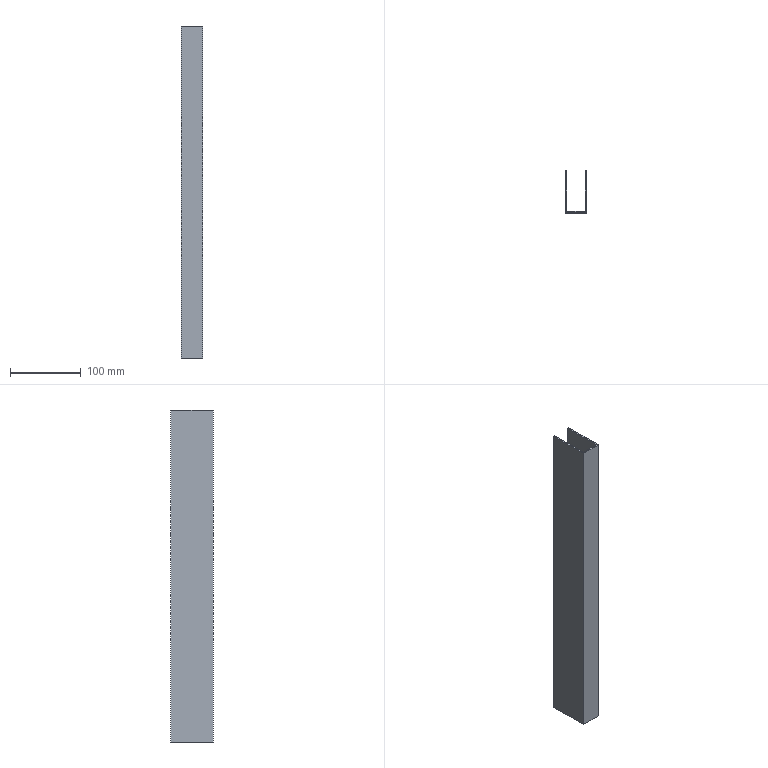Part | SolidWorks | features Extrusion 1, Shell 1 | 1 solid | 10 faces | box 30 x 60 x 470 mm | volume 137240 mm3 | plane 10
STEP:
#1=CARTESIAN_POINT('',(13.,30.,235.));
#2=VERTEX_POINT('',#1);
#3=CARTESIAN_POINT('',(13.,30.,-235.));
#4=VERTEX_POINT('',#3);
#5=CARTESIAN_POINT('',(13.,30.,235.));
#6=DIRECTION('',(0.,0.,-1.));
#7=VECTOR('',#6,1000.);
#8=LINE('',#5,#7);
#9=EDGE_CURVE('',#2,#4,#8,.T.);
#10=ORIENTED_EDGE('',*,*,#9,.F.);
#11=CARTESIAN_POINT('',(15.,30.,235.));
#12=VERTEX_POINT('',#11);
#13=CARTESIAN_POINT('',(-15.,30.,235.));
#14=DIRECTION('',(-1.,0.,0.));
#15=VECTOR('',#14,1000.);
#16=LINE('',#13,#15);
#17=EDGE_CURVE('',#12,#2,#16,.T.);
#18=ORIENTED_EDGE('',*,*,#17,.F.);
#19=CARTESIAN_POINT('',(15.,30.,-235.));
#20=VERTEX_POINT('',#19);
#21=CARTESIAN_POINT('',(15.,30.,235.));
#22=DIRECTION('',(0.,0.,-1.));
#23=VECTOR('',#22,1000.);
#24=LINE('',#21,#23);
#25=EDGE_CURVE('',#12,#20,#24,.T.);
#26=ORIENTED_EDGE('',*,*,#25,.T.);
#27=CARTESIAN_POINT('',(-15.,30.,-235.));
#28=DIRECTION('',(-1.,0.,0.));
#29=VECTOR('',#28,1000.);
#30=LINE('',#27,#29);
#31=EDGE_CURVE('',#20,#4,#30,.T.);
#32=ORIENTED_EDGE('',*,*,#31,.T.);
#33=EDGE_LOOP('',(#10,#18,#26,#32));
#34=FACE_OUTER_BOUND('',#33,.T.);
#35=CARTESIAN_POINT('',(-15.,30.,235.));
#36=DIRECTION('',(0.,-1.,0.));
#37=DIRECTION('',(0.,0.,-1.));
#38=AXIS2_PLACEMENT_3D('',#35,#36,#37);
#39=PLANE('',#38);
#40=ADVANCED_FACE('',(#34),#39,.F.);
#41=CARTESIAN_POINT('',(13.,-28.,235.));
#42=VERTEX_POINT('',#41);
#43=CARTESIAN_POINT('',(13.,0.,235.));
#44=DIRECTION('',(0.,1.,0.));
#45=VECTOR('',#44,1000.);
#46=LINE('',#43,#45);
#47=EDGE_CURVE('',#42,#2,#46,.T.);
#48=ORIENTED_EDGE('',*,*,#47,.F.);
#49=CARTESIAN_POINT('',(-13.,-28.,235.));
#50=VERTEX_POINT('',#49);
#51=CARTESIAN_POINT('',(0.,-28.,235.));
#52=DIRECTION('',(1.,0.,0.));
#53=VECTOR('',#52,1000.);
#54=LINE('',#51,#53);
#55=EDGE_CURVE('',#50,#42,#54,.T.);
#56=ORIENTED_EDGE('',*,*,#55,.F.);
#57=CARTESIAN_POINT('',(-13.,30.,235.));
#58=VERTEX_POINT('',#57);
#59=CARTESIAN_POINT('',(-13.,0.,235.));
#60=DIRECTION('',(0.,-1.,0.));
#61=VECTOR('',#60,1000.);
#62=LINE('',#59,#61);
#63=EDGE_CURVE('',#58,#50,#62,.T.);
#64=ORIENTED_EDGE('',*,*,#63,.F.);
#65=CARTESIAN_POINT('',(-15.,30.,235.));
#66=VERTEX_POINT('',#65);
#67=CARTESIAN_POINT('',(-15.,30.,235.));
#68=DIRECTION('',(-1.,0.,0.));
#69=VECTOR('',#68,1000.);
#70=LINE('',#67,#69);
#71=EDGE_CURVE('',#58,#66,#70,.T.);
#72=ORIENTED_EDGE('',*,*,#71,.T.);
#73=CARTESIAN_POINT('',(-15.,-30.,235.));
#74=VERTEX_POINT('',#73);
#75=CARTESIAN_POINT('',(-15.,-30.,235.));
#76=DIRECTION('',(0.,-1.,0.));
#77=VECTOR('',#76,1000.);
#78=LINE('',#75,#77);
#79=EDGE_CURVE('',#66,#74,#78,.T.);
#80=ORIENTED_EDGE('',*,*,#79,.T.);
#81=CARTESIAN_POINT('',(15.,-30.,235.));
#82=VERTEX_POINT('',#81);
#83=CARTESIAN_POINT('',(-15.,-30.,235.));
#84=DIRECTION('',(1.,0.,0.));
#85=VECTOR('',#84,1000.);
#86=LINE('',#83,#85);
#87=EDGE_CURVE('',#74,#82,#86,.T.);
#88=ORIENTED_EDGE('',*,*,#87,.T.);
#89=CARTESIAN_POINT('',(15.,-30.,235.));
#90=DIRECTION('',(0.,1.,0.));
#91=VECTOR('',#90,1000.);
#92=LINE('',#89,#91);
#93=EDGE_CURVE('',#82,#12,#92,.T.);
#94=ORIENTED_EDGE('',*,*,#93,.T.);
#95=ORIENTED_EDGE('',*,*,#17,.T.);
#96=EDGE_LOOP('',(#48,#56,#64,#72,#80,#88,#94,#95));
#97=FACE_OUTER_BOUND('',#96,.T.);
#98=CARTESIAN_POINT('',(0.,0.,235.));
#99=DIRECTION('',(0.,0.,-1.));
#100=DIRECTION('',(-1.,0.,0.));
#101=AXIS2_PLACEMENT_3D('',#98,#99,#100);
#102=PLANE('',#101);
#103=ADVANCED_FACE('',(#97),#102,.F.);
#104=CARTESIAN_POINT('',(-13.,-28.,-235.));
#105=VERTEX_POINT('',#104);
#106=CARTESIAN_POINT('',(13.,-28.,-235.));
#107=VERTEX_POINT('',#106);
#108=CARTESIAN_POINT('',(0.,-28.,-235.));
#109=DIRECTION('',(1.,0.,0.));
#110=VECTOR('',#109,1000.);
#111=LINE('',#108,#110);
#112=EDGE_CURVE('',#105,#107,#111,.T.);
#113=ORIENTED_EDGE('',*,*,#112,.T.);
#114=CARTESIAN_POINT('',(13.,0.,-235.));
#115=DIRECTION('',(0.,1.,0.));
#116=VECTOR('',#115,1000.);
#117=LINE('',#114,#116);
#118=EDGE_CURVE('',#107,#4,#117,.T.);
#119=ORIENTED_EDGE('',*,*,#118,.T.);
#120=ORIENTED_EDGE('',*,*,#31,.F.);
#121=CARTESIAN_POINT('',(15.,-30.,-235.));
#122=VERTEX_POINT('',#121);
#123=CARTESIAN_POINT('',(15.,-30.,-235.));
#124=DIRECTION('',(0.,1.,0.));
#125=VECTOR('',#124,1000.);
#126=LINE('',#123,#125);
#127=EDGE_CURVE('',#122,#20,#126,.T.);
#128=ORIENTED_EDGE('',*,*,#127,.F.);
#129=CARTESIAN_POINT('',(-15.,-30.,-235.));
#130=VERTEX_POINT('',#129);
#131=CARTESIAN_POINT('',(-15.,-30.,-235.));
#132=DIRECTION('',(1.,0.,0.));
#133=VECTOR('',#132,1000.);
#134=LINE('',#131,#133);
#135=EDGE_CURVE('',#130,#122,#134,.T.);
#136=ORIENTED_EDGE('',*,*,#135,.F.);
#137=CARTESIAN_POINT('',(-15.,30.,-235.));
#138=VERTEX_POINT('',#137);
#139=CARTESIAN_POINT('',(-15.,-30.,-235.));
#140=DIRECTION('',(0.,-1.,0.));
#141=VECTOR('',#140,1000.);
#142=LINE('',#139,#141);
#143=EDGE_CURVE('',#138,#130,#142,.T.);
#144=ORIENTED_EDGE('',*,*,#143,.F.);
#145=CARTESIAN_POINT('',(-13.,30.,-235.));
#146=VERTEX_POINT('',#145);
#147=CARTESIAN_POINT('',(-15.,30.,-235.));
#148=DIRECTION('',(-1.,0.,0.));
#149=VECTOR('',#148,1000.);
#150=LINE('',#147,#149);
#151=EDGE_CURVE('',#146,#138,#150,.T.);
#152=ORIENTED_EDGE('',*,*,#151,.F.);
#153=CARTESIAN_POINT('',(-13.,0.,-235.));
#154=DIRECTION('',(0.,-1.,0.));
#155=VECTOR('',#154,1000.);
#156=LINE('',#153,#155);
#157=EDGE_CURVE('',#146,#105,#156,.T.);
#158=ORIENTED_EDGE('',*,*,#157,.T.);
#159=EDGE_LOOP('',(#113,#119,#120,#128,#136,#144,#152,#158));
#160=FACE_OUTER_BOUND('',#159,.T.);
#161=CARTESIAN_POINT('',(0.,0.,-235.));
#162=DIRECTION('',(0.,0.,-1.));
#163=DIRECTION('',(-1.,0.,0.));
#164=AXIS2_PLACEMENT_3D('',#161,#162,#163);
#165=PLANE('',#164);
#166=ADVANCED_FACE('',(#160),#165,.T.);
#167=ORIENTED_EDGE('',*,*,#127,.T.);
#168=ORIENTED_EDGE('',*,*,#25,.F.);
#169=ORIENTED_EDGE('',*,*,#93,.F.);
#170=CARTESIAN_POINT('',(15.,-30.,235.));
#171=DIRECTION('',(0.,0.,-1.));
#172=VECTOR('',#171,1000.);
#173=LINE('',#170,#172);
#174=EDGE_CURVE('',#82,#122,#173,.T.);
#175=ORIENTED_EDGE('',*,*,#174,.T.);
#176=EDGE_LOOP('',(#167,#168,#169,#175));
#177=FACE_OUTER_BOUND('',#176,.T.);
#178=CARTESIAN_POINT('',(15.,-30.,235.));
#179=DIRECTION('',(-1.,0.,0.));
#180=DIRECTION('',(0.,0.,1.));
#181=AXIS2_PLACEMENT_3D('',#178,#179,#180);
#182=PLANE('',#181);
#183=ADVANCED_FACE('',(#177),#182,.F.);
#184=ORIENTED_EDGE('',*,*,#71,.F.);
#185=CARTESIAN_POINT('',(-13.,30.,235.));
#186=DIRECTION('',(0.,0.,-1.));
#187=VECTOR('',#186,1000.);
#188=LINE('',#185,#187);
#189=EDGE_CURVE('',#58,#146,#188,.T.);
#190=ORIENTED_EDGE('',*,*,#189,.T.);
#191=ORIENTED_EDGE('',*,*,#151,.T.);
#192=CARTESIAN_POINT('',(-15.,30.,235.));
#193=DIRECTION('',(0.,0.,-1.));
#194=VECTOR('',#193,1000.);
#195=LINE('',#192,#194);
#196=EDGE_CURVE('',#66,#138,#195,.T.);
#197=ORIENTED_EDGE('',*,*,#196,.F.);
#198=EDGE_LOOP('',(#184,#190,#191,#197));
#199=FACE_OUTER_BOUND('',#198,.T.);
#200=CARTESIAN_POINT('',(-15.,30.,235.));
#201=DIRECTION('',(0.,-1.,0.));
#202=DIRECTION('',(0.,0.,-1.));
#203=AXIS2_PLACEMENT_3D('',#200,#201,#202);
#204=PLANE('',#203);
#205=ADVANCED_FACE('',(#199),#204,.F.);
#206=ORIENTED_EDGE('',*,*,#143,.T.);
#207=CARTESIAN_POINT('',(-15.,-30.,235.));
#208=DIRECTION('',(0.,0.,-1.));
#209=VECTOR('',#208,1000.);
#210=LINE('',#207,#209);
#211=EDGE_CURVE('',#74,#130,#210,.T.);
#212=ORIENTED_EDGE('',*,*,#211,.F.);
#213=ORIENTED_EDGE('',*,*,#79,.F.);
#214=ORIENTED_EDGE('',*,*,#196,.T.);
#215=EDGE_LOOP('',(#206,#212,#213,#214));
#216=FACE_OUTER_BOUND('',#215,.T.);
#217=CARTESIAN_POINT('',(-15.,-30.,235.));
#218=DIRECTION('',(1.,0.,0.));
#219=DIRECTION('',(0.,0.,-1.));
#220=AXIS2_PLACEMENT_3D('',#217,#218,#219);
#221=PLANE('',#220);
#222=ADVANCED_FACE('',(#216),#221,.F.);
#223=ORIENTED_EDGE('',*,*,#135,.T.);
#224=ORIENTED_EDGE('',*,*,#174,.F.);
#225=ORIENTED_EDGE('',*,*,#87,.F.);
#226=ORIENTED_EDGE('',*,*,#211,.T.);
#227=EDGE_LOOP('',(#223,#224,#225,#226));
#228=FACE_OUTER_BOUND('',#227,.T.);
#229=CARTESIAN_POINT('',(-15.,-30.,235.));
#230=DIRECTION('',(0.,1.,0.));
#231=DIRECTION('',(0.,0.,1.));
#232=AXIS2_PLACEMENT_3D('',#229,#230,#231);
#233=PLANE('',#232);
#234=ADVANCED_FACE('',(#228),#233,.F.);
#235=ORIENTED_EDGE('',*,*,#118,.F.);
#236=CARTESIAN_POINT('',(13.,-28.,235.));
#237=DIRECTION('',(0.,0.,-1.));
#238=VECTOR('',#237,1000.);
#239=LINE('',#236,#238);
#240=EDGE_CURVE('',#42,#107,#239,.T.);
#241=ORIENTED_EDGE('',*,*,#240,.F.);
#242=ORIENTED_EDGE('',*,*,#47,.T.);
#243=ORIENTED_EDGE('',*,*,#9,.T.);
#244=EDGE_LOOP('',(#235,#241,#242,#243));
#245=FACE_OUTER_BOUND('',#244,.T.);
#246=CARTESIAN_POINT('',(13.,-30.,235.));
#247=DIRECTION('',(-1.,0.,0.));
#248=DIRECTION('',(0.,0.,1.));
#249=AXIS2_PLACEMENT_3D('',#246,#247,#248);
#250=PLANE('',#249);
#251=ADVANCED_FACE('',(#245),#250,.T.);
#252=ORIENTED_EDGE('',*,*,#157,.F.);
#253=ORIENTED_EDGE('',*,*,#189,.F.);
#254=ORIENTED_EDGE('',*,*,#63,.T.);
#255=CARTESIAN_POINT('',(-13.,-28.,235.));
#256=DIRECTION('',(0.,0.,-1.));
#257=VECTOR('',#256,1000.);
#258=LINE('',#255,#257);
#259=EDGE_CURVE('',#50,#105,#258,.T.);
#260=ORIENTED_EDGE('',*,*,#259,.T.);
#261=EDGE_LOOP('',(#252,#253,#254,#260));
#262=FACE_OUTER_BOUND('',#261,.T.);
#263=CARTESIAN_POINT('',(-13.,-30.,235.));
#264=DIRECTION('',(1.,0.,0.));
#265=DIRECTION('',(0.,0.,-1.));
#266=AXIS2_PLACEMENT_3D('',#263,#264,#265);
#267=PLANE('',#266);
#268=ADVANCED_FACE('',(#262),#267,.T.);
#269=ORIENTED_EDGE('',*,*,#112,.F.);
#270=ORIENTED_EDGE('',*,*,#259,.F.);
#271=ORIENTED_EDGE('',*,*,#55,.T.);
#272=ORIENTED_EDGE('',*,*,#240,.T.);
#273=EDGE_LOOP('',(#269,#270,#271,#272));
#274=FACE_OUTER_BOUND('',#273,.T.);
#275=CARTESIAN_POINT('',(-15.,-28.,235.));
#276=DIRECTION('',(0.,1.,0.));
#277=DIRECTION('',(0.,0.,1.));
#278=AXIS2_PLACEMENT_3D('',#275,#276,#277);
#279=PLANE('',#278);
#280=ADVANCED_FACE('',(#274),#279,.T.);
#281=CLOSED_SHELL('',(#40,#103,#166,#183,#205,#222,#234,#251,#268,#280));
#282=MANIFOLD_SOLID_BREP('',#281);
#283=CARTESIAN_POINT('',(0.,0.,0.));
#284=DIRECTION('',(0.,0.,1.));
#285=DIRECTION('',(1.,0.,0.));
#286=AXIS2_PLACEMENT_3D('',#283,#284,#285);
#287=(LENGTH_UNIT()NAMED_UNIT(*)SI_UNIT(.MILLI.,.METRE.));
#288=UNCERTAINTY_MEASURE_WITH_UNIT(LENGTH_MEASURE(0.00001),#287,'','');
#289=(NAMED_UNIT(*)PLANE_ANGLE_UNIT()SI_UNIT($,.RADIAN.));
#290=(NAMED_UNIT(*)SI_UNIT($,.STERADIAN.)SOLID_ANGLE_UNIT());
#291=(GEOMETRIC_REPRESENTATION_CONTEXT(3)GLOBAL_UNCERTAINTY_ASSIGNED_CONTEXT((#288))GLOBAL_UNIT_ASSIGNED_CONTEXT((#287,#289,#290))REPRESENTATION_CONTEXT('',''));
#292=ADVANCED_BREP_SHAPE_REPRESENTATION('',(#282,#286),#291);